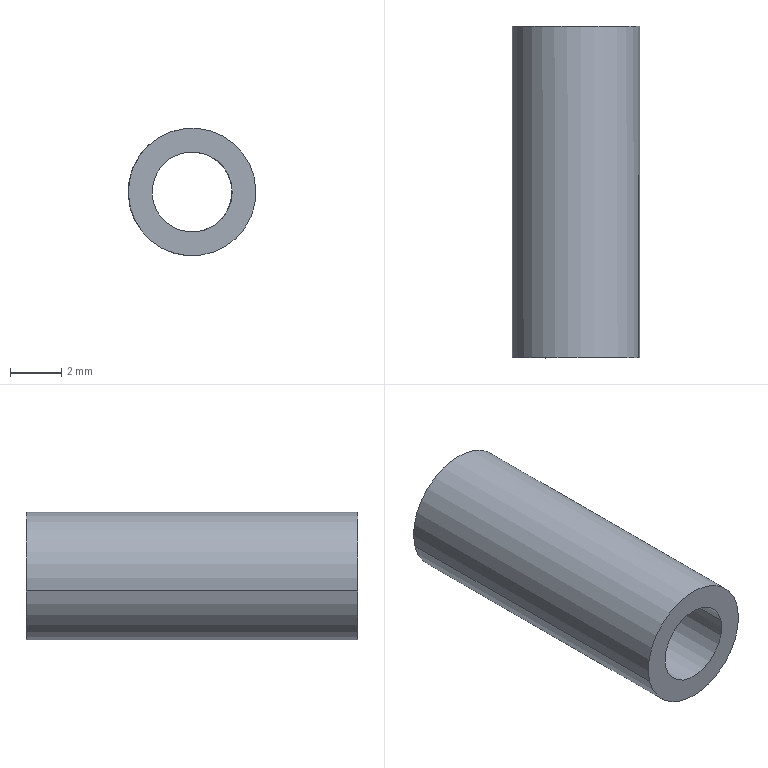Part | SolidWorks | features BaseBody 1 | 1 solid | 6 faces | box 5.012 x 13.005 x 5 mm | volume 154.586 mm3 | cylinder 4 | plane 2 | commonest cylinder face diameters 3.14 x2 5 x2
STEP:
#1=CARTESIAN_POINT('',(343.478,393.966,107.288));
#2=VERTEX_POINT('',#1);
#3=CARTESIAN_POINT('',(340.426,393.963,106.551));
#4=VERTEX_POINT('',#3);
#5=CARTESIAN_POINT('',(341.952,393.964,106.919));
#6=DIRECTION('',(0.0009599,-1.,0.));
#7=DIRECTION('',(-0.9721,-0.0009331,-0.2347));
#8=AXIS2_PLACEMENT_3D('',#5,#6,#7);
#9=CIRCLE('',#8,1.57);
#10=EDGE_CURVE('',#2,#4,#9,.T.);
#11=ORIENTED_EDGE('',*,*,#10,.F.);
#12=CARTESIAN_POINT('',(343.49,380.966,107.288));
#13=VERTEX_POINT('',#12);
#14=CARTESIAN_POINT('',(343.478,393.966,107.288));
#15=DIRECTION('',(0.0009599,-1.,0.));
#16=VECTOR('',#15,1000.);
#17=LINE('',#14,#16);
#18=EDGE_CURVE('',#2,#13,#17,.T.);
#19=ORIENTED_EDGE('',*,*,#18,.T.);
#20=CARTESIAN_POINT('',(340.438,380.963,106.551));
#21=VERTEX_POINT('',#20);
#22=CARTESIAN_POINT('',(341.964,380.964,106.919));
#23=DIRECTION('',(-0.0009599,1.,0.));
#24=DIRECTION('',(0.9721,0.0009331,0.2347));
#25=AXIS2_PLACEMENT_3D('',#22,#23,#24);
#26=CIRCLE('',#25,1.57);
#27=EDGE_CURVE('',#21,#13,#26,.T.);
#28=ORIENTED_EDGE('',*,*,#27,.F.);
#29=CARTESIAN_POINT('',(340.426,393.963,106.551));
#30=DIRECTION('',(0.0009599,-1.,0.));
#31=VECTOR('',#30,1000.);
#32=LINE('',#29,#31);
#33=EDGE_CURVE('',#4,#21,#32,.T.);
#34=ORIENTED_EDGE('',*,*,#33,.F.);
#35=EDGE_LOOP('',(#11,#19,#28,#34));
#36=FACE_OUTER_BOUND('',#35,.T.);
#37=CARTESIAN_POINT('',(341.952,393.964,106.919));
#38=DIRECTION('',(0.0009599,-1.,0.));
#39=DIRECTION('',(-0.9721,-0.0009331,-0.2347));
#40=AXIS2_PLACEMENT_3D('',#37,#38,#39);
#41=CYLINDRICAL_SURFACE('',#40,1.57);
#42=ADVANCED_FACE('',(#36),#41,.F.);
#43=CARTESIAN_POINT('',(344.382,393.966,107.506));
#44=VERTEX_POINT('',#43);
#45=CARTESIAN_POINT('',(339.522,393.962,106.332));
#46=VERTEX_POINT('',#45);
#47=CARTESIAN_POINT('',(341.952,393.964,106.919));
#48=DIRECTION('',(-0.0009599,1.,0.));
#49=DIRECTION('',(0.9721,0.0009331,0.2347));
#50=AXIS2_PLACEMENT_3D('',#47,#48,#49);
#51=CIRCLE('',#50,2.5);
#52=EDGE_CURVE('',#44,#46,#51,.T.);
#53=ORIENTED_EDGE('',*,*,#52,.F.);
#54=CARTESIAN_POINT('',(344.394,380.966,107.506));
#55=VERTEX_POINT('',#54);
#56=CARTESIAN_POINT('',(344.382,393.966,107.506));
#57=DIRECTION('',(0.0009599,-1.,0.));
#58=VECTOR('',#57,1000.);
#59=LINE('',#56,#58);
#60=EDGE_CURVE('',#44,#55,#59,.T.);
#61=ORIENTED_EDGE('',*,*,#60,.T.);
#62=CARTESIAN_POINT('',(339.534,380.962,106.332));
#63=VERTEX_POINT('',#62);
#64=CARTESIAN_POINT('',(341.964,380.964,106.919));
#65=DIRECTION('',(0.0009599,-1.,0.));
#66=DIRECTION('',(0.9721,0.0009331,0.2347));
#67=AXIS2_PLACEMENT_3D('',#64,#65,#66);
#68=CIRCLE('',#67,2.5);
#69=EDGE_CURVE('',#63,#55,#68,.T.);
#70=ORIENTED_EDGE('',*,*,#69,.F.);
#71=CARTESIAN_POINT('',(339.522,393.962,106.332));
#72=DIRECTION('',(0.0009599,-1.,0.));
#73=VECTOR('',#72,1000.);
#74=LINE('',#71,#73);
#75=EDGE_CURVE('',#46,#63,#74,.T.);
#76=ORIENTED_EDGE('',*,*,#75,.F.);
#77=EDGE_LOOP('',(#53,#61,#70,#76));
#78=FACE_OUTER_BOUND('',#77,.T.);
#79=CARTESIAN_POINT('',(341.952,393.964,106.919));
#80=DIRECTION('',(0.0009599,-1.,0.));
#81=DIRECTION('',(-0.9721,-0.0009331,-0.2347));
#82=AXIS2_PLACEMENT_3D('',#79,#80,#81);
#83=CYLINDRICAL_SURFACE('',#82,2.5);
#84=ADVANCED_FACE('',(#78),#83,.T.);
#85=ORIENTED_EDGE('',*,*,#27,.T.);
#86=CARTESIAN_POINT('',(341.964,380.964,106.919));
#87=DIRECTION('',(-0.0009599,1.,0.));
#88=DIRECTION('',(0.9721,0.0009331,0.2347));
#89=AXIS2_PLACEMENT_3D('',#86,#87,#88);
#90=CIRCLE('',#89,1.57);
#91=EDGE_CURVE('',#13,#21,#90,.T.);
#92=ORIENTED_EDGE('',*,*,#91,.T.);
#93=EDGE_LOOP('',(#85,#92));
#94=FACE_BOUND('',#93,.T.);
#95=ORIENTED_EDGE('',*,*,#69,.T.);
#96=CARTESIAN_POINT('',(341.964,380.964,106.919));
#97=DIRECTION('',(0.0009599,-1.,0.));
#98=DIRECTION('',(0.9721,0.0009331,0.2347));
#99=AXIS2_PLACEMENT_3D('',#96,#97,#98);
#100=CIRCLE('',#99,2.5);
#101=EDGE_CURVE('',#55,#63,#100,.T.);
#102=ORIENTED_EDGE('',*,*,#101,.T.);
#103=EDGE_LOOP('',(#95,#102));
#104=FACE_OUTER_BOUND('',#103,.T.);
#105=CARTESIAN_POINT('',(341.964,380.964,106.919));
#106=DIRECTION('',(-0.0009599,1.,0.));
#107=DIRECTION('',(0.,0.,1.));
#108=AXIS2_PLACEMENT_3D('',#105,#106,#107);
#109=PLANE('',#108);
#110=ADVANCED_FACE('',(#94,#104),#109,.F.);
#111=ORIENTED_EDGE('',*,*,#60,.F.);
#112=CARTESIAN_POINT('',(341.952,393.964,106.919));
#113=DIRECTION('',(-0.0009599,1.,0.));
#114=DIRECTION('',(0.9721,0.0009331,0.2347));
#115=AXIS2_PLACEMENT_3D('',#112,#113,#114);
#116=CIRCLE('',#115,2.5);
#117=EDGE_CURVE('',#46,#44,#116,.T.);
#118=ORIENTED_EDGE('',*,*,#117,.F.);
#119=ORIENTED_EDGE('',*,*,#75,.T.);
#120=ORIENTED_EDGE('',*,*,#101,.F.);
#121=EDGE_LOOP('',(#111,#118,#119,#120));
#122=FACE_OUTER_BOUND('',#121,.T.);
#123=CARTESIAN_POINT('',(341.952,393.964,106.919));
#124=DIRECTION('',(0.0009599,-1.,0.));
#125=DIRECTION('',(-0.9721,-0.0009331,-0.2347));
#126=AXIS2_PLACEMENT_3D('',#123,#124,#125);
#127=CYLINDRICAL_SURFACE('',#126,2.5);
#128=ADVANCED_FACE('',(#122),#127,.T.);
#129=CARTESIAN_POINT('',(341.952,393.964,106.919));
#130=DIRECTION('',(0.0009599,-1.,0.));
#131=DIRECTION('',(-0.9721,-0.0009331,-0.2347));
#132=AXIS2_PLACEMENT_3D('',#129,#130,#131);
#133=CIRCLE('',#132,1.57);
#134=EDGE_CURVE('',#4,#2,#133,.T.);
#135=ORIENTED_EDGE('',*,*,#134,.T.);
#136=ORIENTED_EDGE('',*,*,#10,.T.);
#137=EDGE_LOOP('',(#135,#136));
#138=FACE_BOUND('',#137,.T.);
#139=ORIENTED_EDGE('',*,*,#117,.T.);
#140=ORIENTED_EDGE('',*,*,#52,.T.);
#141=EDGE_LOOP('',(#139,#140));
#142=FACE_OUTER_BOUND('',#141,.T.);
#143=CARTESIAN_POINT('',(341.952,393.964,106.919));
#144=DIRECTION('',(-0.0009599,1.,0.));
#145=DIRECTION('',(0.,0.,1.));
#146=AXIS2_PLACEMENT_3D('',#143,#144,#145);
#147=PLANE('',#146);
#148=ADVANCED_FACE('',(#138,#142),#147,.T.);
#149=ORIENTED_EDGE('',*,*,#18,.F.);
#150=ORIENTED_EDGE('',*,*,#134,.F.);
#151=ORIENTED_EDGE('',*,*,#33,.T.);
#152=ORIENTED_EDGE('',*,*,#91,.F.);
#153=EDGE_LOOP('',(#149,#150,#151,#152));
#154=FACE_OUTER_BOUND('',#153,.T.);
#155=CARTESIAN_POINT('',(341.952,393.964,106.919));
#156=DIRECTION('',(0.0009599,-1.,0.));
#157=DIRECTION('',(-0.9721,-0.0009331,-0.2347));
#158=AXIS2_PLACEMENT_3D('',#155,#156,#157);
#159=CYLINDRICAL_SURFACE('',#158,1.57);
#160=ADVANCED_FACE('',(#154),#159,.F.);
#161=CLOSED_SHELL('',(#42,#84,#110,#128,#148,#160));
#162=MANIFOLD_SOLID_BREP('',#161);
#163=CARTESIAN_POINT('',(0.,0.,0.));
#164=DIRECTION('',(0.,0.,1.));
#165=DIRECTION('',(1.,0.,0.));
#166=AXIS2_PLACEMENT_3D('',#163,#164,#165);
#167=(LENGTH_UNIT()NAMED_UNIT(*)SI_UNIT(.MILLI.,.METRE.));
#168=UNCERTAINTY_MEASURE_WITH_UNIT(LENGTH_MEASURE(0.00001),#167,'','');
#169=(NAMED_UNIT(*)PLANE_ANGLE_UNIT()SI_UNIT($,.RADIAN.));
#170=(NAMED_UNIT(*)SI_UNIT($,.STERADIAN.)SOLID_ANGLE_UNIT());
#171=(GEOMETRIC_REPRESENTATION_CONTEXT(3)GLOBAL_UNCERTAINTY_ASSIGNED_CONTEXT((#168))GLOBAL_UNIT_ASSIGNED_CONTEXT((#167,#169,#170))REPRESENTATION_CONTEXT('',''));
#172=ADVANCED_BREP_SHAPE_REPRESENTATION('',(#162,#166),#171);